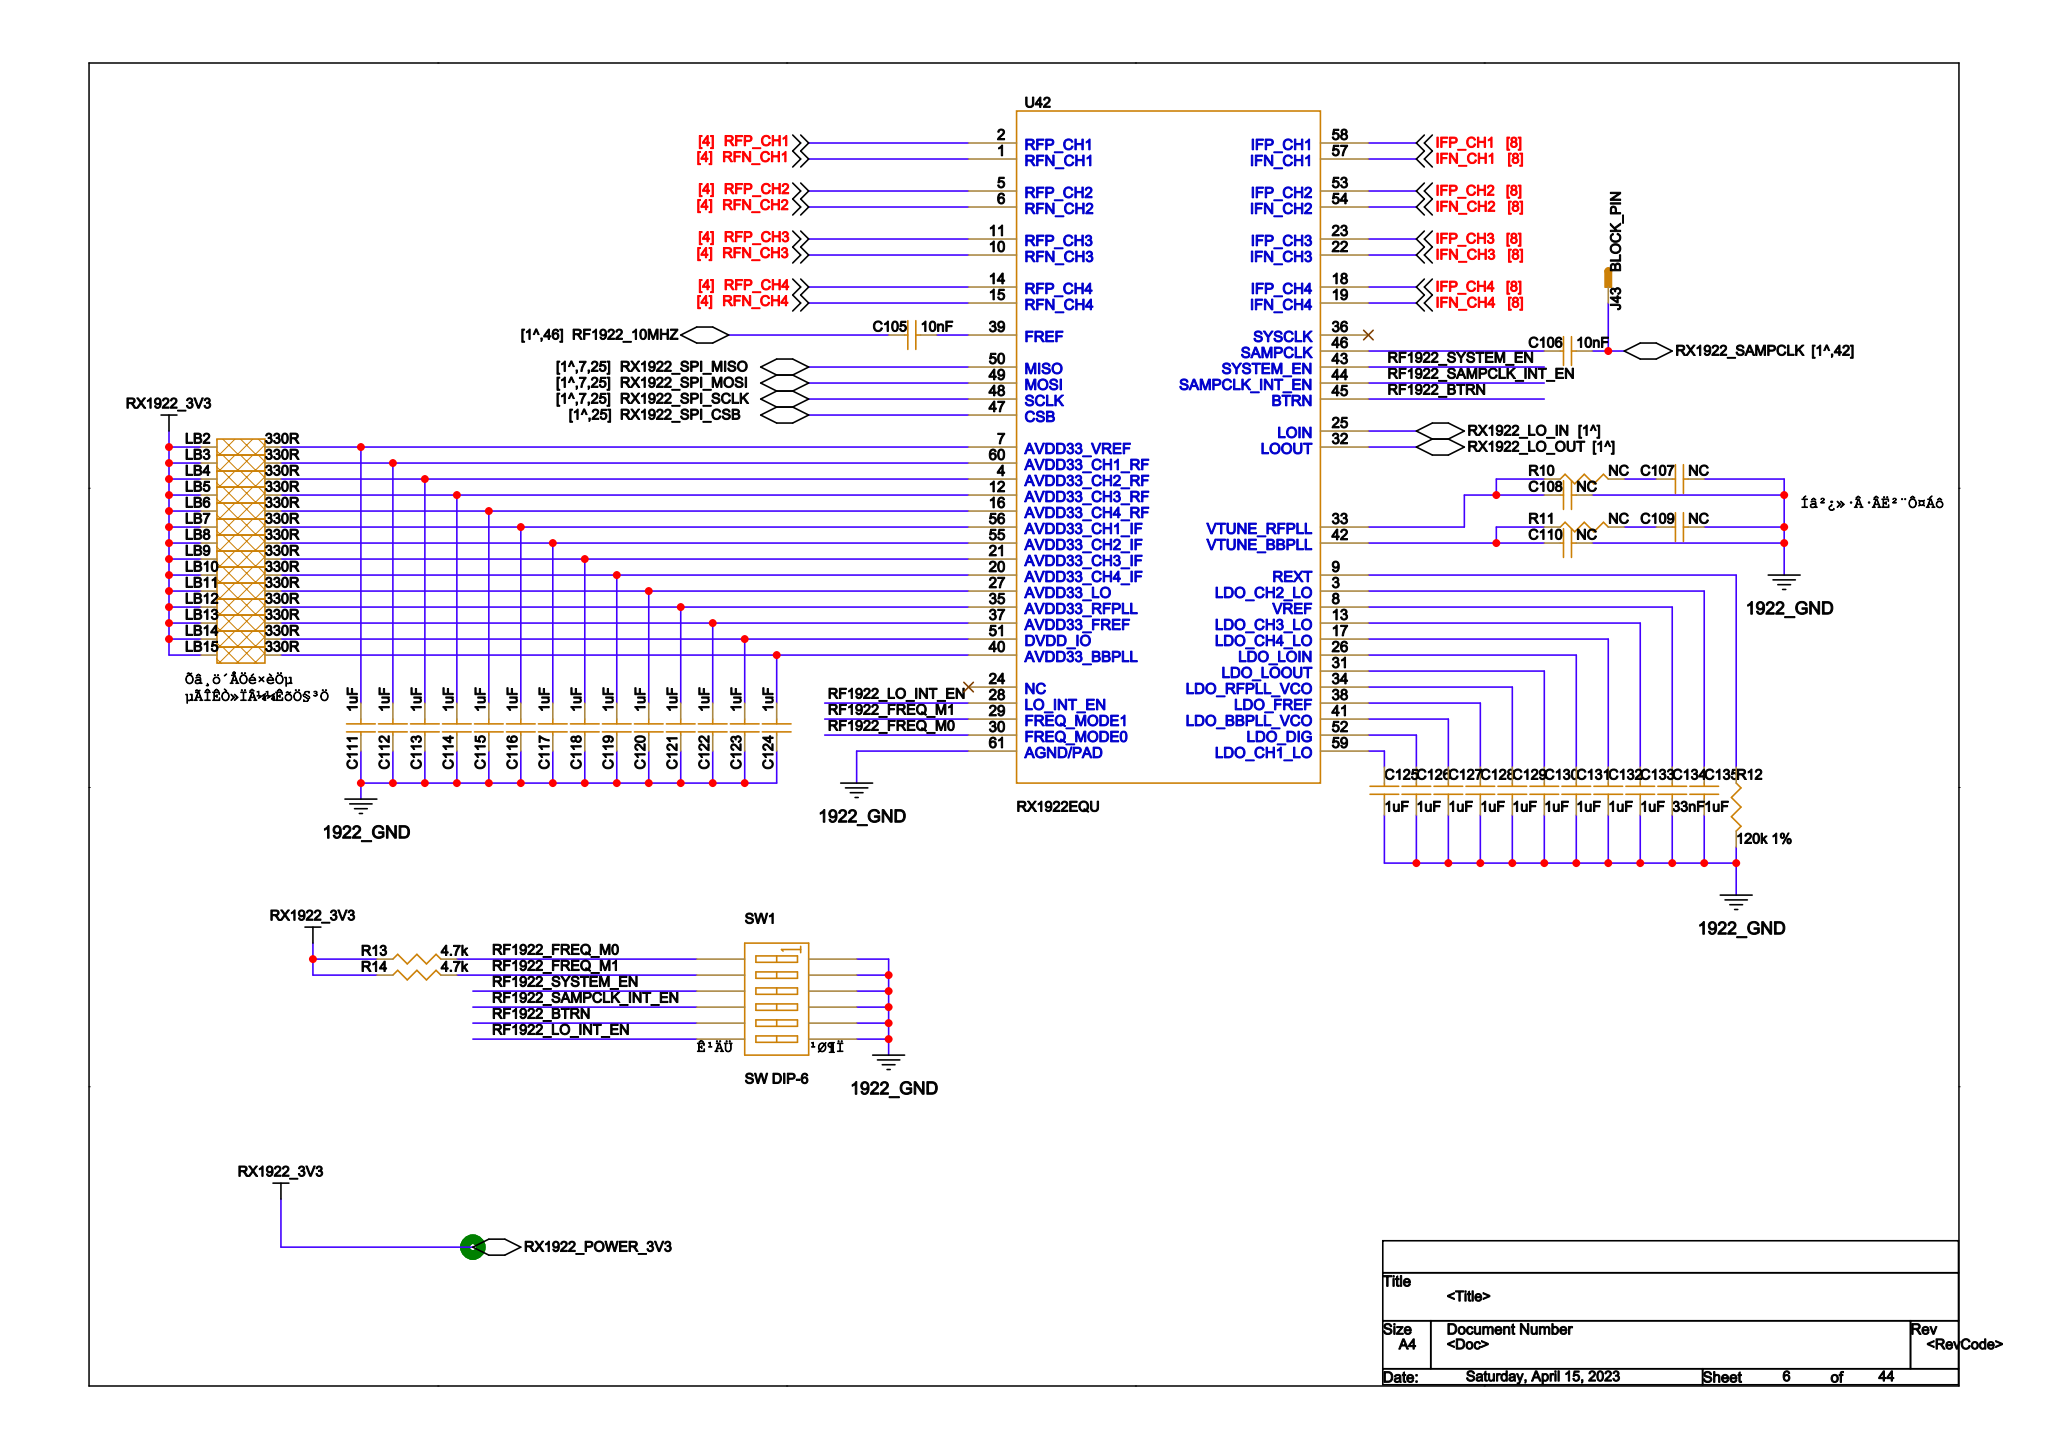Circuit board | Cadence Allegro | 1034 parts | 912 nets | one sheet of the schematic
Parts on this sheet (reference | value | footprint):
C105 | 10nF | C0402
C106 | 10nF | C0402
C107 | NC | C0402
C108 | NC | C0402
C109 | NC | C0402
C110 | NC | C0402
C111 | 1uF | C0402
C112 | 1uF | C0402
C113 | 1uF | C0402
C114 | 1uF | C0402
C115 | 1uF | C0402
C116 | 1uF | C0402
C117 | 1uF | C0402
C118 | 1uF | C0402
C119 | 1uF | C0402
C120 | 1uF | C0402
C121 | 1uF | C0402
C122 | 1uF | C0402
C123 | 1uF | C0402
C124 | 1uF | C0402
C125 | 1uF | C0402
C126 | 1uF | C0402
C127 | 1uF | C0402
C128 | 1uF | C0402
C129 | 1uF | C0402
C130 | 1uF | C0402
C131 | 1uF | C0402
C132 | 1uF | C0402
C133 | 1uF | C0402
C134 | 33nF | C0402
C135 | 1uF | C0402
J43 | BLOCK_PIN | B_PIN_SMD
LB2 | 330R | LB0402
LB3 | 330R | LB0402
LB4 | 330R | LB0402
LB5 | 330R | LB0402
LB6 | 330R | LB0402
LB7 | 330R | LB0402
LB8 | 330R | LB0402
LB9 | 330R | LB0402
LB10 | 330R | LB0402
LB11 | 330R | LB0402
LB12 | 330R | LB0402
LB13 | 330R | LB0402
LB14 | 330R | LB0402
LB15 | 330R | LB0402
R10 | NC | R0402
R11 | NC | R0402
R12 | 120k 1% | R0402
R13 | 4.7k | R0402
SW1 | SW DIP-6 | SW_6_SOP
U42 | RX1922EQU | RX1922_QFN60
Nets of these parts (net: part-pin ...):
N188110: C106-2 J43-1
1922_GND: C107-2 C108-2 C109-2 C110-2 C111-1 C112-1 C113-1 C114-1 C115-1 C116-1 C117-1 C118-1 C119-1 C120-1 C121-1 C122-1 C123-1 C124-1 C125-2 C126-2 C127-2 C128-2 C129-2 C130-2 C131-2 C132-2 C133-2 C134-2 C135-2 R12-2 SW1-7 SW1-8 SW1-9 SW1-10 SW1-11 SW1-12 U42-61
PWR1922_3V3_1: LB2-1 LB3-1 LB4-1 LB5-1 LB6-1 LB7-1 LB8-1 LB9-1 LB10-1 LB11-1 LB12-1 LB13-1 LB14-1 LB15-1 R13-1
N424630_D1: C119-2 LB10-2 U42-20
N424634_D1: C120-2 LB11-2 U42-27
N424606_D1: C121-2 LB12-2 U42-35
N424610_D1: C122-2 LB13-2 U42-37
N424588_D1: C123-2 LB14-2 U42-51
N424576_D1: C124-2 LB15-2 U42-40
N424726_D1: C111-2 LB2-2 U42-7
N424730_D1: C112-2 LB3-2 U42-60
N424678_D1: C113-2 LB4-2 U42-4
N424682_D1: C114-2 LB5-2 U42-12
N424686_D1: C115-2 LB6-2 U42-16
N424690_D1: C116-2 LB7-2 U42-56
N424694_D1: C117-2 LB8-2 U42-55
N424698_D1: C118-2 LB9-2 U42-21
N244712: C105-1
N426726_D1: C105-2 U42-39
N426273_D1: C106-1 U42-46
N425592_D1: C107-1 R10-2
N425584_D1: C108-1 R10-1 U42-33
N425372_D1: C109-1 R11-2
N425300_D1: C110-1 R11-1 U42-42
N382314_D1: C125-1 U42-59
N382275_D1: C126-1 U42-52
N382268_D1: C127-1 U42-41
N382255_D1: C128-1 U42-38
N382242_D1: C129-1 U42-34
N382235_D1: C130-1 U42-31
N382222_D1: C131-1 U42-26
N382215_D1: C132-1 U42-17
N382202_D1: C133-1 U42-13
N382176_D1: C135-1 U42-3
N382189_D1: C134-1 U42-8
RF1922_FREQ_M0_D1: R13-2 SW1-1 U42-30
RF1922_FREQ_M1_D1: SW1-2 U42-29
N382169_D1: R12-1 U42-9
RF1922_SYSTEM_EN_D1: SW1-3 U42-43
RF1922_SAMPCLK_INT_EN_D1: SW1-4 U42-44
RF1922_BTRN_D1: SW1-5 U42-45
RF1922_LO_INT_EN_D1: SW1-6 U42-28